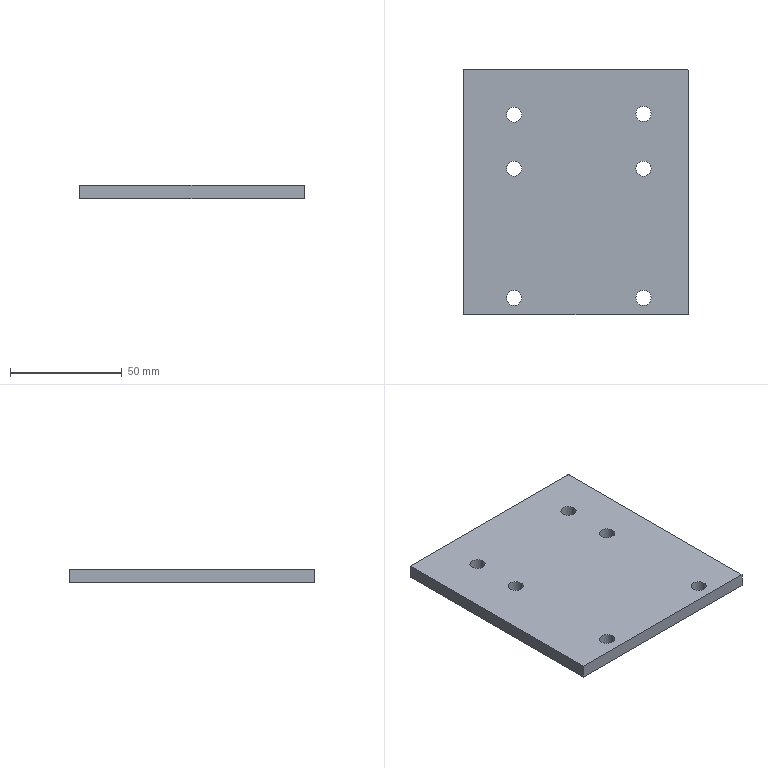Part | STEP file | Mirrored pad plate | 1 solid | 31 faces | box 100.5 x 110 x 6 mm | volume 64996 mm3 | cylinder 13 | cone 12 | plane 6 | commonest cylinder face diameters 6.8 x12 1 x1
STEP:
#1=CARTESIAN_POINT('',(238.4,0.,-5.375));
#2=VERTEX_POINT('',#1);
#3=CARTESIAN_POINT('',(231.6,0.,-5.375));
#4=VERTEX_POINT('',#3);
#5=CARTESIAN_POINT('',(235.,0.,-5.375));
#6=DIRECTION('',(0.,0.,1.));
#7=DIRECTION('',(1.,0.,0.));
#8=AXIS2_PLACEMENT_3D('',#5,#6,#7);
#9=CIRCLE('',#8,3.4);
#10=EDGE_CURVE('',#2,#4,#9,.T.);
#11=ORIENTED_EDGE('',*,*,#10,.T.);
#12=CARTESIAN_POINT('',(230.975,0.,-6.));
#13=VERTEX_POINT('',#12);
#14=CARTESIAN_POINT('',(230.975,0.,-6.));
#15=DIRECTION('',(-0.7071,0.,-0.7071));
#16=VECTOR('',#15,1000.);
#17=LINE('',#14,#16);
#18=EDGE_CURVE('',#4,#13,#17,.T.);
#19=ORIENTED_EDGE('',*,*,#18,.T.);
#20=CARTESIAN_POINT('',(239.025,0.,-6.));
#21=VERTEX_POINT('',#20);
#22=CARTESIAN_POINT('',(235.,0.,-6.));
#23=DIRECTION('',(0.,0.,1.));
#24=DIRECTION('',(1.,0.,0.));
#25=AXIS2_PLACEMENT_3D('',#22,#23,#24);
#26=CIRCLE('',#25,4.025);
#27=EDGE_CURVE('',#21,#13,#26,.T.);
#28=ORIENTED_EDGE('',*,*,#27,.F.);
#29=CARTESIAN_POINT('',(239.025,0.,-6.));
#30=DIRECTION('',(0.7071,0.,-0.7071));
#31=VECTOR('',#30,1000.);
#32=LINE('',#29,#31);
#33=EDGE_CURVE('',#2,#21,#32,.T.);
#34=ORIENTED_EDGE('',*,*,#33,.F.);
#35=EDGE_LOOP('',(#11,#19,#28,#34));
#36=FACE_OUTER_BOUND('',#35,.T.);
#37=CARTESIAN_POINT('',(235.,0.,-6.));
#38=DIRECTION('',(0.,0.,-1.));
#39=DIRECTION('',(1.,0.,0.));
#40=AXIS2_PLACEMENT_3D('',#37,#38,#39);
#41=CONICAL_SURFACE('',#40,4.025,0.7854);
#42=ADVANCED_FACE('',(#36),#41,.F.);
#43=CARTESIAN_POINT('',(231.6,0.,0.));
#44=VERTEX_POINT('',#43);
#45=CARTESIAN_POINT('',(238.4,0.,0.));
#46=VERTEX_POINT('',#45);
#47=CARTESIAN_POINT('',(235.,0.,0.));
#48=DIRECTION('',(0.,0.,-1.));
#49=DIRECTION('',(-1.,0.,0.));
#50=AXIS2_PLACEMENT_3D('',#47,#48,#49);
#51=CIRCLE('',#50,3.4);
#52=EDGE_CURVE('',#44,#46,#51,.T.);
#53=ORIENTED_EDGE('',*,*,#52,.F.);
#54=CARTESIAN_POINT('',(231.6,0.,-6.));
#55=DIRECTION('',(0.,0.,-1.));
#56=VECTOR('',#55,1000.);
#57=LINE('',#54,#56);
#58=EDGE_CURVE('',#44,#4,#57,.T.);
#59=ORIENTED_EDGE('',*,*,#58,.T.);
#60=ORIENTED_EDGE('',*,*,#10,.F.);
#61=CARTESIAN_POINT('',(238.4,0.,-6.));
#62=DIRECTION('',(0.,0.,-1.));
#63=VECTOR('',#62,1000.);
#64=LINE('',#61,#63);
#65=EDGE_CURVE('',#46,#2,#64,.T.);
#66=ORIENTED_EDGE('',*,*,#65,.F.);
#67=EDGE_LOOP('',(#53,#59,#60,#66));
#68=FACE_OUTER_BOUND('',#67,.T.);
#69=CARTESIAN_POINT('',(235.,0.,-6.));
#70=DIRECTION('',(0.,0.,-1.));
#71=DIRECTION('',(1.,0.,0.));
#72=AXIS2_PLACEMENT_3D('',#69,#70,#71);
#73=CYLINDRICAL_SURFACE('',#72,3.4);
#74=ADVANCED_FACE('',(#68),#73,.F.);
#75=CARTESIAN_POINT('',(238.4,-24.5,-5.375));
#76=VERTEX_POINT('',#75);
#77=CARTESIAN_POINT('',(231.6,-24.5,-5.375));
#78=VERTEX_POINT('',#77);
#79=CARTESIAN_POINT('',(235.,-24.5,-5.375));
#80=DIRECTION('',(0.,0.,1.));
#81=DIRECTION('',(1.,0.,0.));
#82=AXIS2_PLACEMENT_3D('',#79,#80,#81);
#83=CIRCLE('',#82,3.4);
#84=EDGE_CURVE('',#76,#78,#83,.T.);
#85=ORIENTED_EDGE('',*,*,#84,.T.);
#86=CARTESIAN_POINT('',(230.975,-24.5,-6.));
#87=VERTEX_POINT('',#86);
#88=CARTESIAN_POINT('',(230.975,-24.5,-6.));
#89=DIRECTION('',(-0.7071,0.,-0.7071));
#90=VECTOR('',#89,1000.);
#91=LINE('',#88,#90);
#92=EDGE_CURVE('',#78,#87,#91,.T.);
#93=ORIENTED_EDGE('',*,*,#92,.T.);
#94=CARTESIAN_POINT('',(239.025,-24.5,-6.));
#95=VERTEX_POINT('',#94);
#96=CARTESIAN_POINT('',(235.,-24.5,-6.));
#97=DIRECTION('',(0.,0.,1.));
#98=DIRECTION('',(1.,0.,0.));
#99=AXIS2_PLACEMENT_3D('',#96,#97,#98);
#100=CIRCLE('',#99,4.025);
#101=EDGE_CURVE('',#95,#87,#100,.T.);
#102=ORIENTED_EDGE('',*,*,#101,.F.);
#103=CARTESIAN_POINT('',(239.025,-24.5,-6.));
#104=DIRECTION('',(0.7071,0.,-0.7071));
#105=VECTOR('',#104,1000.);
#106=LINE('',#103,#105);
#107=EDGE_CURVE('',#76,#95,#106,.T.);
#108=ORIENTED_EDGE('',*,*,#107,.F.);
#109=EDGE_LOOP('',(#85,#93,#102,#108));
#110=FACE_OUTER_BOUND('',#109,.T.);
#111=CARTESIAN_POINT('',(235.,-24.5,-6.));
#112=DIRECTION('',(0.,0.,-1.));
#113=DIRECTION('',(1.,0.,0.));
#114=AXIS2_PLACEMENT_3D('',#111,#112,#113);
#115=CONICAL_SURFACE('',#114,4.025,0.7854);
#116=ADVANCED_FACE('',(#110),#115,.F.);
#117=CARTESIAN_POINT('',(231.6,-24.5,0.));
#118=VERTEX_POINT('',#117);
#119=CARTESIAN_POINT('',(238.4,-24.5,0.));
#120=VERTEX_POINT('',#119);
#121=CARTESIAN_POINT('',(235.,-24.5,0.));
#122=DIRECTION('',(0.,0.,-1.));
#123=DIRECTION('',(-1.,0.,0.));
#124=AXIS2_PLACEMENT_3D('',#121,#122,#123);
#125=CIRCLE('',#124,3.4);
#126=EDGE_CURVE('',#118,#120,#125,.T.);
#127=ORIENTED_EDGE('',*,*,#126,.F.);
#128=CARTESIAN_POINT('',(231.6,-24.5,-6.));
#129=DIRECTION('',(0.,0.,-1.));
#130=VECTOR('',#129,1000.);
#131=LINE('',#128,#130);
#132=EDGE_CURVE('',#118,#78,#131,.T.);
#133=ORIENTED_EDGE('',*,*,#132,.T.);
#134=ORIENTED_EDGE('',*,*,#84,.F.);
#135=CARTESIAN_POINT('',(238.4,-24.5,-6.));
#136=DIRECTION('',(0.,0.,-1.));
#137=VECTOR('',#136,1000.);
#138=LINE('',#135,#137);
#139=EDGE_CURVE('',#120,#76,#138,.T.);
#140=ORIENTED_EDGE('',*,*,#139,.F.);
#141=EDGE_LOOP('',(#127,#133,#134,#140));
#142=FACE_OUTER_BOUND('',#141,.T.);
#143=CARTESIAN_POINT('',(235.,-24.5,-6.));
#144=DIRECTION('',(0.,0.,-1.));
#145=DIRECTION('',(1.,0.,0.));
#146=AXIS2_PLACEMENT_3D('',#143,#144,#145);
#147=CYLINDRICAL_SURFACE('',#146,3.4);
#148=ADVANCED_FACE('',(#142),#147,.F.);
#149=CARTESIAN_POINT('',(238.4,-82.5,-5.375));
#150=VERTEX_POINT('',#149);
#151=CARTESIAN_POINT('',(231.6,-82.5,-5.375));
#152=VERTEX_POINT('',#151);
#153=CARTESIAN_POINT('',(235.,-82.5,-5.375));
#154=DIRECTION('',(0.,0.,1.));
#155=DIRECTION('',(1.,0.,0.));
#156=AXIS2_PLACEMENT_3D('',#153,#154,#155);
#157=CIRCLE('',#156,3.4);
#158=EDGE_CURVE('',#150,#152,#157,.T.);
#159=ORIENTED_EDGE('',*,*,#158,.T.);
#160=CARTESIAN_POINT('',(230.975,-82.5,-6.));
#161=VERTEX_POINT('',#160);
#162=CARTESIAN_POINT('',(230.975,-82.5,-6.));
#163=DIRECTION('',(-0.7071,0.,-0.7071));
#164=VECTOR('',#163,1000.);
#165=LINE('',#162,#164);
#166=EDGE_CURVE('',#152,#161,#165,.T.);
#167=ORIENTED_EDGE('',*,*,#166,.T.);
#168=CARTESIAN_POINT('',(239.025,-82.5,-6.));
#169=VERTEX_POINT('',#168);
#170=CARTESIAN_POINT('',(235.,-82.5,-6.));
#171=DIRECTION('',(0.,0.,1.));
#172=DIRECTION('',(1.,0.,0.));
#173=AXIS2_PLACEMENT_3D('',#170,#171,#172);
#174=CIRCLE('',#173,4.025);
#175=EDGE_CURVE('',#169,#161,#174,.T.);
#176=ORIENTED_EDGE('',*,*,#175,.F.);
#177=CARTESIAN_POINT('',(239.025,-82.5,-6.));
#178=DIRECTION('',(0.7071,0.,-0.7071));
#179=VECTOR('',#178,1000.);
#180=LINE('',#177,#179);
#181=EDGE_CURVE('',#150,#169,#180,.T.);
#182=ORIENTED_EDGE('',*,*,#181,.F.);
#183=EDGE_LOOP('',(#159,#167,#176,#182));
#184=FACE_OUTER_BOUND('',#183,.T.);
#185=CARTESIAN_POINT('',(235.,-82.5,-6.));
#186=DIRECTION('',(0.,0.,-1.));
#187=DIRECTION('',(1.,0.,0.));
#188=AXIS2_PLACEMENT_3D('',#185,#186,#187);
#189=CONICAL_SURFACE('',#188,4.025,0.7854);
#190=ADVANCED_FACE('',(#184),#189,.F.);
#191=CARTESIAN_POINT('',(231.6,-82.5,0.));
#192=VERTEX_POINT('',#191);
#193=CARTESIAN_POINT('',(238.4,-82.5,0.));
#194=VERTEX_POINT('',#193);
#195=CARTESIAN_POINT('',(235.,-82.5,0.));
#196=DIRECTION('',(0.,0.,-1.));
#197=DIRECTION('',(-1.,0.,0.));
#198=AXIS2_PLACEMENT_3D('',#195,#196,#197);
#199=CIRCLE('',#198,3.4);
#200=EDGE_CURVE('',#192,#194,#199,.T.);
#201=ORIENTED_EDGE('',*,*,#200,.F.);
#202=CARTESIAN_POINT('',(231.6,-82.5,-6.));
#203=DIRECTION('',(0.,0.,-1.));
#204=VECTOR('',#203,1000.);
#205=LINE('',#202,#204);
#206=EDGE_CURVE('',#192,#152,#205,.T.);
#207=ORIENTED_EDGE('',*,*,#206,.T.);
#208=ORIENTED_EDGE('',*,*,#158,.F.);
#209=CARTESIAN_POINT('',(238.4,-82.5,-6.));
#210=DIRECTION('',(0.,0.,-1.));
#211=VECTOR('',#210,1000.);
#212=LINE('',#209,#211);
#213=EDGE_CURVE('',#194,#150,#212,.T.);
#214=ORIENTED_EDGE('',*,*,#213,.F.);
#215=EDGE_LOOP('',(#201,#207,#208,#214));
#216=FACE_OUTER_BOUND('',#215,.T.);
#217=CARTESIAN_POINT('',(235.,-82.5,-6.));
#218=DIRECTION('',(0.,0.,-1.));
#219=DIRECTION('',(1.,0.,0.));
#220=AXIS2_PLACEMENT_3D('',#217,#218,#219);
#221=CYLINDRICAL_SURFACE('',#220,3.4);
#222=ADVANCED_FACE('',(#216),#221,.F.);
#223=CARTESIAN_POINT('',(180.4,-82.5,-5.375));
#224=VERTEX_POINT('',#223);
#225=CARTESIAN_POINT('',(173.6,-82.5,-5.375));
#226=VERTEX_POINT('',#225);
#227=CARTESIAN_POINT('',(177.,-82.5,-5.375));
#228=DIRECTION('',(0.,0.,1.));
#229=DIRECTION('',(1.,0.,0.));
#230=AXIS2_PLACEMENT_3D('',#227,#228,#229);
#231=CIRCLE('',#230,3.4);
#232=EDGE_CURVE('',#224,#226,#231,.T.);
#233=ORIENTED_EDGE('',*,*,#232,.T.);
#234=CARTESIAN_POINT('',(172.975,-82.5,-6.));
#235=VERTEX_POINT('',#234);
#236=CARTESIAN_POINT('',(172.975,-82.5,-6.));
#237=DIRECTION('',(-0.7071,0.,-0.7071));
#238=VECTOR('',#237,1000.);
#239=LINE('',#236,#238);
#240=EDGE_CURVE('',#226,#235,#239,.T.);
#241=ORIENTED_EDGE('',*,*,#240,.T.);
#242=CARTESIAN_POINT('',(181.025,-82.5,-6.));
#243=VERTEX_POINT('',#242);
#244=CARTESIAN_POINT('',(177.,-82.5,-6.));
#245=DIRECTION('',(0.,0.,1.));
#246=DIRECTION('',(1.,0.,0.));
#247=AXIS2_PLACEMENT_3D('',#244,#245,#246);
#248=CIRCLE('',#247,4.025);
#249=EDGE_CURVE('',#243,#235,#248,.T.);
#250=ORIENTED_EDGE('',*,*,#249,.F.);
#251=CARTESIAN_POINT('',(181.025,-82.5,-6.));
#252=DIRECTION('',(0.7071,0.,-0.7071));
#253=VECTOR('',#252,1000.);
#254=LINE('',#251,#253);
#255=EDGE_CURVE('',#224,#243,#254,.T.);
#256=ORIENTED_EDGE('',*,*,#255,.F.);
#257=EDGE_LOOP('',(#233,#241,#250,#256));
#258=FACE_OUTER_BOUND('',#257,.T.);
#259=CARTESIAN_POINT('',(177.,-82.5,-6.));
#260=DIRECTION('',(0.,0.,-1.));
#261=DIRECTION('',(1.,0.,0.));
#262=AXIS2_PLACEMENT_3D('',#259,#260,#261);
#263=CONICAL_SURFACE('',#262,4.025,0.7854);
#264=ADVANCED_FACE('',(#258),#263,.F.);
#265=CARTESIAN_POINT('',(173.6,-82.5,0.));
#266=VERTEX_POINT('',#265);
#267=CARTESIAN_POINT('',(180.4,-82.5,0.));
#268=VERTEX_POINT('',#267);
#269=CARTESIAN_POINT('',(177.,-82.5,0.));
#270=DIRECTION('',(0.,0.,-1.));
#271=DIRECTION('',(-1.,0.,0.));
#272=AXIS2_PLACEMENT_3D('',#269,#270,#271);
#273=CIRCLE('',#272,3.4);
#274=EDGE_CURVE('',#266,#268,#273,.T.);
#275=ORIENTED_EDGE('',*,*,#274,.F.);
#276=CARTESIAN_POINT('',(173.6,-82.5,-6.));
#277=DIRECTION('',(0.,0.,-1.));
#278=VECTOR('',#277,1000.);
#279=LINE('',#276,#278);
#280=EDGE_CURVE('',#266,#226,#279,.T.);
#281=ORIENTED_EDGE('',*,*,#280,.T.);
#282=ORIENTED_EDGE('',*,*,#232,.F.);
#283=CARTESIAN_POINT('',(180.4,-82.5,-6.));
#284=DIRECTION('',(0.,0.,-1.));
#285=VECTOR('',#284,1000.);
#286=LINE('',#283,#285);
#287=EDGE_CURVE('',#268,#224,#286,.T.);
#288=ORIENTED_EDGE('',*,*,#287,.F.);
#289=EDGE_LOOP('',(#275,#281,#282,#288));
#290=FACE_OUTER_BOUND('',#289,.T.);
#291=CARTESIAN_POINT('',(177.,-82.5,-6.));
#292=DIRECTION('',(0.,0.,-1.));
#293=DIRECTION('',(1.,0.,0.));
#294=AXIS2_PLACEMENT_3D('',#291,#292,#293);
#295=CYLINDRICAL_SURFACE('',#294,3.4);
#296=ADVANCED_FACE('',(#290),#295,.F.);
#297=CARTESIAN_POINT('',(180.4,-24.5,-5.375));
#298=VERTEX_POINT('',#297);
#299=CARTESIAN_POINT('',(173.6,-24.5,-5.375));
#300=VERTEX_POINT('',#299);
#301=CARTESIAN_POINT('',(177.,-24.5,-5.375));
#302=DIRECTION('',(0.,0.,1.));
#303=DIRECTION('',(1.,0.,0.));
#304=AXIS2_PLACEMENT_3D('',#301,#302,#303);
#305=CIRCLE('',#304,3.4);
#306=EDGE_CURVE('',#298,#300,#305,.T.);
#307=ORIENTED_EDGE('',*,*,#306,.T.);
#308=CARTESIAN_POINT('',(172.975,-24.5,-6.));
#309=VERTEX_POINT('',#308);
#310=CARTESIAN_POINT('',(172.975,-24.5,-6.));
#311=DIRECTION('',(-0.7071,0.,-0.7071));
#312=VECTOR('',#311,1000.);
#313=LINE('',#310,#312);
#314=EDGE_CURVE('',#300,#309,#313,.T.);
#315=ORIENTED_EDGE('',*,*,#314,.T.);
#316=CARTESIAN_POINT('',(181.025,-24.5,-6.));
#317=VERTEX_POINT('',#316);
#318=CARTESIAN_POINT('',(177.,-24.5,-6.));
#319=DIRECTION('',(0.,0.,1.));
#320=DIRECTION('',(1.,0.,0.));
#321=AXIS2_PLACEMENT_3D('',#318,#319,#320);
#322=CIRCLE('',#321,4.025);
#323=EDGE_CURVE('',#317,#309,#322,.T.);
#324=ORIENTED_EDGE('',*,*,#323,.F.);
#325=CARTESIAN_POINT('',(181.025,-24.5,-6.));
#326=DIRECTION('',(0.7071,0.,-0.7071));
#327=VECTOR('',#326,1000.);
#328=LINE('',#325,#327);
#329=EDGE_CURVE('',#298,#317,#328,.T.);
#330=ORIENTED_EDGE('',*,*,#329,.F.);
#331=EDGE_LOOP('',(#307,#315,#324,#330));
#332=FACE_OUTER_BOUND('',#331,.T.);
#333=CARTESIAN_POINT('',(177.,-24.5,-6.));
#334=DIRECTION('',(0.,0.,-1.));
#335=DIRECTION('',(1.,0.,0.));
#336=AXIS2_PLACEMENT_3D('',#333,#334,#335);
#337=CONICAL_SURFACE('',#336,4.025,0.7854);
#338=ADVANCED_FACE('',(#332),#337,.F.);
#339=CARTESIAN_POINT('',(173.6,-24.5,0.));
#340=VERTEX_POINT('',#339);
#341=CARTESIAN_POINT('',(180.4,-24.5,0.));
#342=VERTEX_POINT('',#341);
#343=CARTESIAN_POINT('',(177.,-24.5,0.));
#344=DIRECTION('',(0.,0.,-1.));
#345=DIRECTION('',(-1.,0.,0.));
#346=AXIS2_PLACEMENT_3D('',#343,#344,#345);
#347=CIRCLE('',#346,3.4);
#348=EDGE_CURVE('',#340,#342,#347,.T.);
#349=ORIENTED_EDGE('',*,*,#348,.F.);
#350=CARTESIAN_POINT('',(173.6,-24.5,-6.));
#351=DIRECTION('',(0.,0.,-1.));
#352=VECTOR('',#351,1000.);
#353=LINE('',#350,#352);
#354=EDGE_CURVE('',#340,#300,#353,.T.);
#355=ORIENTED_EDGE('',*,*,#354,.T.);
#356=ORIENTED_EDGE('',*,*,#306,.F.);
#357=CARTESIAN_POINT('',(180.4,-24.5,-6.));
#358=DIRECTION('',(0.,0.,-1.));
#359=VECTOR('',#358,1000.);
#360=LINE('',#357,#359);
#361=EDGE_CURVE('',#342,#298,#360,.T.);
#362=ORIENTED_EDGE('',*,*,#361,.F.);
#363=EDGE_LOOP('',(#349,#355,#356,#362));
#364=FACE_OUTER_BOUND('',#363,.T.);
#365=CARTESIAN_POINT('',(177.,-24.5,-6.));
#366=DIRECTION('',(0.,0.,-1.));
#367=DIRECTION('',(1.,0.,0.));
#368=AXIS2_PLACEMENT_3D('',#365,#366,#367);
#369=CYLINDRICAL_SURFACE('',#368,3.4);
#370=ADVANCED_FACE('',(#364),#369,.F.);
#371=CARTESIAN_POINT('',(180.4,-0.3,-5.375));
#372=VERTEX_POINT('',#371);
#373=CARTESIAN_POINT('',(173.6,-0.3,-5.375));
#374=VERTEX_POINT('',#373);
#375=CARTESIAN_POINT('',(177.,-0.3,-5.375));
#376=DIRECTION('',(0.,0.,1.));
#377=DIRECTION('',(1.,0.,0.));
#378=AXIS2_PLACEMENT_3D('',#375,#376,#377);
#379=CIRCLE('',#378,3.4);
#380=EDGE_CURVE('',#372,#374,#379,.T.);
#381=ORIENTED_EDGE('',*,*,#380,.T.);
#382=CARTESIAN_POINT('',(172.975,-0.3,-6.));
#383=VERTEX_POINT('',#382);
#384=CARTESIAN_POINT('',(172.975,-0.3,-6.));
#385=DIRECTION('',(-0.7071,0.,-0.7071));
#386=VECTOR('',#385,1000.);
#387=LINE('',#384,#386);
#388=EDGE_CURVE('',#374,#383,#387,.T.);
#389=ORIENTED_EDGE('',*,*,#388,.T.);
#390=CARTESIAN_POINT('',(181.025,-0.3,-6.));
#391=VERTEX_POINT('',#390);
#392=CARTESIAN_POINT('',(177.,-0.3,-6.));
#393=DIRECTION('',(0.,0.,1.));
#394=DIRECTION('',(1.,0.,0.));
#395=AXIS2_PLACEMENT_3D('',#392,#393,#394);
#396=CIRCLE('',#395,4.025);
#397=EDGE_CURVE('',#391,#383,#396,.T.);
#398=ORIENTED_EDGE('',*,*,#397,.F.);
#399=CARTESIAN_POINT('',(181.025,-0.3,-6.));
#400=DIRECTION('',(0.7071,0.,-0.7071));
#401=VECTOR('',#400,1000.);
#402=LINE('',#399,#401);
#403=EDGE_CURVE('',#372,#391,#402,.T.);
#404=ORIENTED_EDGE('',*,*,#403,.F.);
#405=EDGE_LOOP('',(#381,#389,#398,#404));
#406=FACE_OUTER_BOUND('',#405,.T.);
#407=CARTESIAN_POINT('',(177.,-0.3,-6.));
#408=DIRECTION('',(0.,0.,-1.));
#409=DIRECTION('',(1.,0.,0.));
#410=AXIS2_PLACEMENT_3D('',#407,#408,#409);
#411=CONICAL_SURFACE('',#410,4.025,0.7854);
#412=ADVANCED_FACE('',(#406),#411,.F.);
#413=CARTESIAN_POINT('',(173.6,-0.3,0.));
#414=VERTEX_POINT('',#413);
#415=CARTESIAN_POINT('',(180.4,-0.3,0.));
#416=VERTEX_POINT('',#415);
#417=CARTESIAN_POINT('',(177.,-0.3,0.));
#418=DIRECTION('',(0.,0.,-1.));
#419=DIRECTION('',(-1.,0.,0.));
#420=AXIS2_PLACEMENT_3D('',#417,#418,#419);
#421=CIRCLE('',#420,3.4);
#422=EDGE_CURVE('',#414,#416,#421,.T.);
#423=ORIENTED_EDGE('',*,*,#422,.F.);
#424=CARTESIAN_POINT('',(173.6,-0.3,-6.));
#425=DIRECTION('',(0.,0.,-1.));
#426=VECTOR('',#425,1000.);
#427=LINE('',#424,#426);
#428=EDGE_CURVE('',#414,#374,#427,.T.);
#429=ORIENTED_EDGE('',*,*,#428,.T.);
#430=ORIENTED_EDGE('',*,*,#380,.F.);
#431=CARTESIAN_POINT('',(180.4,-0.3,-6.));
#432=DIRECTION('',(0.,0.,-1.));
#433=VECTOR('',#432,1000.);
#434=LINE('',#431,#433);
#435=EDGE_CURVE('',#416,#372,#434,.T.);
#436=ORIENTED_EDGE('',*,*,#435,.F.);
#437=EDGE_LOOP('',(#423,#429,#430,#436));
#438=FACE_OUTER_BOUND('',#437,.T.);
#439=CARTESIAN_POINT('',(177.,-0.3,-6.));
#440=DIRECTION('',(0.,0.,-1.));
#441=DIRECTION('',(1.,0.,0.));
#442=AXIS2_PLACEMENT_3D('',#439,#440,#441);
#443=CYLINDRICAL_SURFACE('',#442,3.4);
#444=ADVANCED_FACE('',(#438),#443,.F.);
#445=CARTESIAN_POINT('',(154.5,20.,-6.));
#446=VERTEX_POINT('',#445);
#447=CARTESIAN_POINT('',(154.5,-90.,-6.));
#448=VERTEX_POINT('',#447);
#449=CARTESIAN_POINT('',(154.5,20.,-6.));
#450=DIRECTION('',(0.,-1.,0.));
#451=VECTOR('',#450,1000.);
#452=LINE('',#449,#451);
#453=EDGE_CURVE('',#446,#448,#452,.T.);
#454=ORIENTED_EDGE('',*,*,#453,.F.);
#455=CARTESIAN_POINT('',(254.5,20.,-6.));
#456=VERTEX_POINT('',#455);
#457=CARTESIAN_POINT('',(254.5,20.,-6.));
#458=DIRECTION('',(-1.,0.,0.));
#459=VECTOR('',#458,1000.);
#460=LINE('',#457,#459);
#461=EDGE_CURVE('',#456,#446,#460,.T.);
#462=ORIENTED_EDGE('',*,*,#461,.F.);
#463=CARTESIAN_POINT('',(255.,19.5,-6.));
#464=VERTEX_POINT('',#463);
#465=CARTESIAN_POINT('',(254.5,19.5,-6.));
#466=DIRECTION('',(0.,0.,1.));
#467=DIRECTION('',(-1.,0.,0.));
#468=AXIS2_PLACEMENT_3D('',#465,#466,#467);
#469=CIRCLE('',#468,0.5);
#470=EDGE_CURVE('',#464,#456,#469,.T.);
#471=ORIENTED_EDGE('',*,*,#470,.F.);
#472=CARTESIAN_POINT('',(255.,-90.,-6.));
#473=VERTEX_POINT('',#472);
#474=CARTESIAN_POINT('',(255.,19.5,-6.));
#475=DIRECTION('',(0.,1.,0.));
#476=VECTOR('',#475,1000.);
#477=LINE('',#474,#476);
#478=EDGE_CURVE('',#473,#464,#477,.T.);
#479=ORIENTED_EDGE('',*,*,#478,.F.);
#480=CARTESIAN_POINT('',(255.,-90.,-6.));
#481=DIRECTION('',(1.,0.,0.));
#482=VECTOR('',#481,1000.);
#483=LINE('',#480,#482);
#484=EDGE_CURVE('',#448,#473,#483,.T.);
#485=ORIENTED_EDGE('',*,*,#484,.F.);
#486=EDGE_LOOP('',(#454,#462,#471,#479,#485));
#487=FACE_OUTER_BOUND('',#486,.T.);
#488=ORIENTED_EDGE('',*,*,#397,.T.);
#489=CARTESIAN_POINT('',(177.,-0.3,-6.));
#490=DIRECTION('',(0.,0.,1.));
#491=DIRECTION('',(1.,0.,0.));
#492=AXIS2_PLACEMENT_3D('',#489,#490,#491);
#493=CIRCLE('',#492,4.025);
#494=EDGE_CURVE('',#383,#391,#493,.T.);
#495=ORIENTED_EDGE('',*,*,#494,.T.);
#496=EDGE_LOOP('',(#488,#495));
#497=FACE_BOUND('',#496,.T.);
#498=ORIENTED_EDGE('',*,*,#323,.T.);
#499=CARTESIAN_POINT('',(177.,-24.5,-6.));
#500=DIRECTION('',(0.,0.,1.));
#501=DIRECTION('',(1.,0.,0.));
#502=AXIS2_PLACEMENT_3D('',#499,#500,#501);
#503=CIRCLE('',#502,4.025);
#504=EDGE_CURVE('',#309,#317,#503,.T.);
#505=ORIENTED_EDGE('',*,*,#504,.T.);
#506=EDGE_LOOP('',(#498,#505));
#507=FACE_BOUND('',#506,.T.);
#508=ORIENTED_EDGE('',*,*,#249,.T.);
#509=CARTESIAN_POINT('',(177.,-82.5,-6.));
#510=DIRECTION('',(0.,0.,1.));
#511=DIRECTION('',(1.,0.,0.));
#512=AXIS2_PLACEMENT_3D('',#509,#510,#511);
#513=CIRCLE('',#512,4.025);
#514=EDGE_CURVE('',#235,#243,#513,.T.);
#515=ORIENTED_EDGE('',*,*,#514,.T.);
#516=EDGE_LOOP('',(#508,#515));
#517=FACE_BOUND('',#516,.T.);
#518=ORIENTED_EDGE('',*,*,#175,.T.);
#519=CARTESIAN_POINT('',(235.,-82.5,-6.));
#520=DIRECTION('',(0.,0.,1.));
#521=DIRECTION('',(1.,0.,0.));
#522=AXIS2_PLACEMENT_3D('',#519,#520,#521);
#523=CIRCLE('',#522,4.025);
#524=EDGE_CURVE('',#161,#169,#523,.T.);
#525=ORIENTED_EDGE('',*,*,#524,.T.);
#526=EDGE_LOOP('',(#518,#525));
#527=FACE_BOUND('',#526,.T.);
#528=ORIENTED_EDGE('',*,*,#101,.T.);
#529=CARTESIAN_POINT('',(235.,-24.5,-6.));
#530=DIRECTION('',(0.,0.,1.));
#531=DIRECTION('',(1.,0.,0.));
#532=AXIS2_PLACEMENT_3D('',#529,#530,#531);
#533=CIRCLE('',#532,4.025);
#534=EDGE_CURVE('',#87,#95,#533,.T.);
#535=ORIENTED_EDGE('',*,*,#534,.T.);
#536=EDGE_LOOP('',(#528,#535));
#537=FACE_BOUND('',#536,.T.);
#538=ORIENTED_EDGE('',*,*,#27,.T.);
#539=CARTESIAN_POINT('',(235.,0.,-6.));
#540=DIRECTION('',(0.,0.,1.));
#541=DIRECTION('',(1.,0.,0.));
#542=AXIS2_PLACEMENT_3D('',#539,#540,#541);
#543=CIRCLE('',#542,4.025);
#544=EDGE_CURVE('',#13,#21,#543,.T.);
#545=ORIENTED_EDGE('',*,*,#544,.T.);
#546=EDGE_LOOP('',(#538,#545));
#547=FACE_BOUND('',#546,.T.);
#548=CARTESIAN_POINT('',(254.5,19.5,-6.));
#549=DIRECTION('',(0.,0.,1.));
#550=DIRECTION('',(-1.,0.,0.));
#551=AXIS2_PLACEMENT_3D('',#548,#549,#550);
#552=PLANE('',#551);
#553=ADVANCED_FACE('',(#487,#497,#507,#517,#527,#537,#547),#552,.F.);
#554=CARTESIAN_POINT('',(154.5,20.,0.));
#555=VERTEX_POINT('',#554);
#556=CARTESIAN_POINT('',(154.5,-90.,0.));
#557=VERTEX_POINT('',#556);
#558=CARTESIAN_POINT('',(154.5,20.,0.));
#559=DIRECTION('',(0.,-1.,0.));
#560=VECTOR('',#559,1000.);
#561=LINE('',#558,#560);
#562=EDGE_CURVE('',#555,#557,#561,.T.);
#563=ORIENTED_EDGE('',*,*,#562,.F.);
#564=CARTESIAN_POINT('',(154.5,20.,-6.));
#565=DIRECTION('',(0.,0.,1.));
#566=VECTOR('',#565,1000.);
#567=LINE('',#564,#566);
#568=EDGE_CURVE('',#446,#555,#567,.T.);
#569=ORIENTED_EDGE('',*,*,#568,.F.);
#570=ORIENTED_EDGE('',*,*,#453,.T.);
#571=CARTESIAN_POINT('',(154.5,-90.,-6.));
#572=DIRECTION('',(0.,0.,1.));
#573=VECTOR('',#572,1000.);
#574=LINE('',#571,#573);
#575=EDGE_CURVE('',#448,#557,#574,.T.);
#576=ORIENTED_EDGE('',*,*,#575,.T.);
#577=EDGE_LOOP('',(#563,#569,#570,#576));
#578=FACE_OUTER_BOUND('',#577,.T.);
#579=CARTESIAN_POINT('',(154.5,20.,-6.));
#580=DIRECTION('',(1.,0.,0.));
#581=DIRECTION('',(0.,1.,0.));
#582=AXIS2_PLACEMENT_3D('',#579,#580,#581);
#583=PLANE('',#582);
#584=ADVANCED_FACE('',(#578),#583,.F.);
#585=CARTESIAN_POINT('',(255.,-90.,0.));
#586=VERTEX_POINT('',#585);
#587=CARTESIAN_POINT('',(255.,-90.,0.));
#588=DIRECTION('',(1.,0.,0.));
#589=VECTOR('',#588,1000.);
#590=LINE('',#587,#589);
#591=EDGE_CURVE('',#557,#586,#590,.T.);
#592=ORIENTED_EDGE('',*,*,#591,.F.);
#593=ORIENTED_EDGE('',*,*,#575,.F.);
#594=ORIENTED_EDGE('',*,*,#484,.T.);
#595=CARTESIAN_POINT('',(255.,-90.,-6.));
#596=DIRECTION('',(0.,0.,1.));
#597=VECTOR('',#596,1000.);
#598=LINE('',#595,#597);
#599=EDGE_CURVE('',#473,#586,#598,.T.);
#600=ORIENTED_EDGE('',*,*,#599,.T.);
#601=EDGE_LOOP('',(#592,#593,#594,#600));
#602=FACE_OUTER_BOUND('',#601,.T.);
#603=CARTESIAN_POINT('',(255.,-90.,-6.));
#604=DIRECTION('',(0.,1.,0.));
#605=DIRECTION('',(-1.,0.,0.));
#606=AXIS2_PLACEMENT_3D('',#603,#604,#605);
#607=PLANE('',#606);
#608=ADVANCED_FACE('',(#602),#607,.F.);
#609=CARTESIAN_POINT('',(255.,19.5,0.));
#610=VERTEX_POINT('',#609);
#611=CARTESIAN_POINT('',(255.,19.5,0.));
#612=DIRECTION('',(0.,1.,0.));
#613=VECTOR('',#612,1000.);
#614=LINE('',#611,#613);
#615=EDGE_CURVE('',#586,#610,#614,.T.);
#616=ORIENTED_EDGE('',*,*,#615,.F.);
#617=ORIENTED_EDGE('',*,*,#599,.F.);
#618=ORIENTED_EDGE('',*,*,#478,.T.);
#619=CARTESIAN_POINT('',(255.,19.5,-6.));
#620=DIRECTION('',(0.,0.,1.));
#621=VECTOR('',#620,1000.);
#622=LINE('',#619,#621);
#623=EDGE_CURVE('',#464,#610,#622,.T.);
#624=ORIENTED_EDGE('',*,*,#623,.T.);
#625=EDGE_LOOP('',(#616,#617,#618,#624));
#626=FACE_OUTER_BOUND('',#625,.T.);
#627=CARTESIAN_POINT('',(255.,19.5,-6.));
#628=DIRECTION('',(-1.,0.,0.));
#629=DIRECTION('',(0.,0.,-1.));
#630=AXIS2_PLACEMENT_3D('',#627,#628,#629);
#631=PLANE('',#630);
#632=ADVANCED_FACE('',(#626),#631,.F.);
#633=CARTESIAN_POINT('',(254.5,20.,0.));
#634=VERTEX_POINT('',#633);
#635=CARTESIAN_POINT('',(254.5,19.5,0.));
#636=DIRECTION('',(0.,0.,1.));
#637=DIRECTION('',(-1.,0.,0.));
#638=AXIS2_PLACEMENT_3D('',#635,#636,#637);
#639=CIRCLE('',#638,0.5);
#640=EDGE_CURVE('',#610,#634,#639,.T.);
#641=ORIENTED_EDGE('',*,*,#640,.F.);
#642=ORIENTED_EDGE('',*,*,#623,.F.);
#643=ORIENTED_EDGE('',*,*,#470,.T.);
#644=CARTESIAN_POINT('',(254.5,20.,-6.));
#645=DIRECTION('',(0.,0.,1.));
#646=VECTOR('',#645,1000.);
#647=LINE('',#644,#646);
#648=EDGE_CURVE('',#456,#634,#647,.T.);
#649=ORIENTED_EDGE('',*,*,#648,.T.);
#650=EDGE_LOOP('',(#641,#642,#643,#649));
#651=FACE_OUTER_BOUND('',#650,.T.);
#652=CARTESIAN_POINT('',(254.5,19.5,-6.));
#653=DIRECTION('',(0.,0.,1.));
#654=DIRECTION('',(-1.,0.,0.));
#655=AXIS2_PLACEMENT_3D('',#652,#653,#654);
#656=CYLINDRICAL_SURFACE('',#655,0.5);
#657=ADVANCED_FACE('',(#651),#656,.T.);
#658=CARTESIAN_POINT('',(254.5,20.,0.));
#659=DIRECTION('',(-1.,0.,0.));
#660=VECTOR('',#659,1000.);
#661=LINE('',#658,#660);
#662=EDGE_CURVE('',#634,#555,#661,.T.);
#663=ORIENTED_EDGE('',*,*,#662,.F.);
#664=ORIENTED_EDGE('',*,*,#648,.F.);
#665=ORIENTED_EDGE('',*,*,#461,.T.);
#666=ORIENTED_EDGE('',*,*,#568,.T.);
#667=EDGE_LOOP('',(#663,#664,#665,#666));
#668=FACE_OUTER_BOUND('',#667,.T.);
#669=CARTESIAN_POINT('',(254.5,20.,-6.));
#670=DIRECTION('',(0.,-1.,0.));
#671=DIRECTION('',(1.,0.,0.));
#672=AXIS2_PLACEMENT_3D('',#669,#670,#671);
#673=PLANE('',#672);
#674=ADVANCED_FACE('',(#668),#673,.F.);
#675=CARTESIAN_POINT('',(235.,0.,0.));
#676=DIRECTION('',(0.,0.,-1.));
#677=DIRECTION('',(-1.,0.,0.));
#678=AXIS2_PLACEMENT_3D('',#675,#676,#677);
#679=CIRCLE('',#678,3.4);
#680=EDGE_CURVE('',#46,#44,#679,.T.);
#681=ORIENTED_EDGE('',*,*,#680,.T.);
#682=ORIENTED_EDGE('',*,*,#52,.T.);
#683=EDGE_LOOP('',(#681,#682));
#684=FACE_BOUND('',#683,.T.);
#685=CARTESIAN_POINT('',(235.,-24.5,0.));
#686=DIRECTION('',(0.,0.,-1.));
#687=DIRECTION('',(-1.,0.,0.));
#688=AXIS2_PLACEMENT_3D('',#685,#686,#687);
#689=CIRCLE('',#688,3.4);
#690=EDGE_CURVE('',#120,#118,#689,.T.);
#691=ORIENTED_EDGE('',*,*,#690,.T.);
#692=ORIENTED_EDGE('',*,*,#126,.T.);
#693=EDGE_LOOP('',(#691,#692));
#694=FACE_BOUND('',#693,.T.);
#695=CARTESIAN_POINT('',(235.,-82.5,0.));
#696=DIRECTION('',(0.,0.,-1.));
#697=DIRECTION('',(-1.,0.,0.));
#698=AXIS2_PLACEMENT_3D('',#695,#696,#697);
#699=CIRCLE('',#698,3.4);
#700=EDGE_CURVE('',#194,#192,#699,.T.);
#701=ORIENTED_EDGE('',*,*,#700,.T.);
#702=ORIENTED_EDGE('',*,*,#200,.T.);
#703=EDGE_LOOP('',(#701,#702));
#704=FACE_BOUND('',#703,.T.);
#705=CARTESIAN_POINT('',(177.,-82.5,0.));
#706=DIRECTION('',(0.,0.,-1.));
#707=DIRECTION('',(-1.,0.,0.));
#708=AXIS2_PLACEMENT_3D('',#705,#706,#707);
#709=CIRCLE('',#708,3.4);
#710=EDGE_CURVE('',#268,#266,#709,.T.);
#711=ORIENTED_EDGE('',*,*,#710,.T.);
#712=ORIENTED_EDGE('',*,*,#274,.T.);
#713=EDGE_LOOP('',(#711,#712));
#714=FACE_BOUND('',#713,.T.);
#715=CARTESIAN_POINT('',(177.,-24.5,0.));
#716=DIRECTION('',(0.,0.,-1.));
#717=DIRECTION('',(-1.,0.,0.));
#718=AXIS2_PLACEMENT_3D('',#715,#716,#717);
#719=CIRCLE('',#718,3.4);
#720=EDGE_CURVE('',#342,#340,#719,.T.);
#721=ORIENTED_EDGE('',*,*,#720,.T.);
#722=ORIENTED_EDGE('',*,*,#348,.T.);
#723=EDGE_LOOP('',(#721,#722));
#724=FACE_BOUND('',#723,.T.);
#725=CARTESIAN_POINT('',(177.,-0.3,0.));
#726=DIRECTION('',(0.,0.,-1.));
#727=DIRECTION('',(-1.,0.,0.));
#728=AXIS2_PLACEMENT_3D('',#725,#726,#727);
#729=CIRCLE('',#728,3.4);
#730=EDGE_CURVE('',#416,#414,#729,.T.);
#731=ORIENTED_EDGE('',*,*,#730,.T.);
#732=ORIENTED_EDGE('',*,*,#422,.T.);
#733=EDGE_LOOP('',(#731,#732));
#734=FACE_BOUND('',#733,.T.);
#735=ORIENTED_EDGE('',*,*,#562,.T.);
#736=ORIENTED_EDGE('',*,*,#591,.T.);
#737=ORIENTED_EDGE('',*,*,#615,.T.);
#738=ORIENTED_EDGE('',*,*,#640,.T.);
#739=ORIENTED_EDGE('',*,*,#662,.T.);
#740=EDGE_LOOP('',(#735,#736,#737,#738,#739));
#741=FACE_OUTER_BOUND('',#740,.T.);
#742=CARTESIAN_POINT('',(254.5,19.5,0.));
#743=DIRECTION('',(0.,0.,1.));
#744=DIRECTION('',(-1.,0.,0.));
#745=AXIS2_PLACEMENT_3D('',#742,#743,#744);
#746=PLANE('',#745);
#747=ADVANCED_FACE('',(#684,#694,#704,#714,#724,#734,#741),#746,.T.);
#748=ORIENTED_EDGE('',*,*,#428,.F.);
#749=ORIENTED_EDGE('',*,*,#730,.F.);
#750=ORIENTED_EDGE('',*,*,#435,.T.);
#751=CARTESIAN_POINT('',(177.,-0.3,-5.375));
#752=DIRECTION('',(0.,0.,1.));
#753=DIRECTION('',(1.,0.,0.));
#754=AXIS2_PLACEMENT_3D('',#751,#752,#753);
#755=CIRCLE('',#754,3.4);
#756=EDGE_CURVE('',#374,#372,#755,.T.);
#757=ORIENTED_EDGE('',*,*,#756,.F.);
#758=EDGE_LOOP('',(#748,#749,#750,#757));
#759=FACE_OUTER_BOUND('',#758,.T.);
#760=CARTESIAN_POINT('',(177.,-0.3,-6.));
#761=DIRECTION('',(0.,0.,-1.));
#762=DIRECTION('',(1.,0.,0.));
#763=AXIS2_PLACEMENT_3D('',#760,#761,#762);
#764=CYLINDRICAL_SURFACE('',#763,3.4);
#765=ADVANCED_FACE('',(#759),#764,.F.);
#766=ORIENTED_EDGE('',*,*,#388,.F.);
#767=ORIENTED_EDGE('',*,*,#756,.T.);
#768=ORIENTED_EDGE('',*,*,#403,.T.);
#769=ORIENTED_EDGE('',*,*,#494,.F.);
#770=EDGE_LOOP('',(#766,#767,#768,#769));
#771=FACE_OUTER_BOUND('',#770,.T.);
#772=CARTESIAN_POINT('',(177.,-0.3,-6.));
#773=DIRECTION('',(0.,0.,-1.));
#774=DIRECTION('',(1.,0.,0.));
#775=AXIS2_PLACEMENT_3D('',#772,#773,#774);
#776=CONICAL_SURFACE('',#775,4.025,0.7854);
#777=ADVANCED_FACE('',(#771),#776,.F.);
#778=ORIENTED_EDGE('',*,*,#354,.F.);
#779=ORIENTED_EDGE('',*,*,#720,.F.);
#780=ORIENTED_EDGE('',*,*,#361,.T.);
#781=CARTESIAN_POINT('',(177.,-24.5,-5.375));
#782=DIRECTION('',(0.,0.,1.));
#783=DIRECTION('',(1.,0.,0.));
#784=AXIS2_PLACEMENT_3D('',#781,#782,#783);
#785=CIRCLE('',#784,3.4);
#786=EDGE_CURVE('',#300,#298,#785,.T.);
#787=ORIENTED_EDGE('',*,*,#786,.F.);
#788=EDGE_LOOP('',(#778,#779,#780,#787));
#789=FACE_OUTER_BOUND('',#788,.T.);
#790=CARTESIAN_POINT('',(177.,-24.5,-6.));
#791=DIRECTION('',(0.,0.,-1.));
#792=DIRECTION('',(1.,0.,0.));
#793=AXIS2_PLACEMENT_3D('',#790,#791,#792);
#794=CYLINDRICAL_SURFACE('',#793,3.4);
#795=ADVANCED_FACE('',(#789),#794,.F.);
#796=ORIENTED_EDGE('',*,*,#314,.F.);
#797=ORIENTED_EDGE('',*,*,#786,.T.);
#798=ORIENTED_EDGE('',*,*,#329,.T.);
#799=ORIENTED_EDGE('',*,*,#504,.F.);
#800=EDGE_LOOP('',(#796,#797,#798,#799));
#801=FACE_OUTER_BOUND('',#800,.T.);
#802=CARTESIAN_POINT('',(177.,-24.5,-6.));
#803=DIRECTION('',(0.,0.,-1.));
#804=DIRECTION('',(1.,0.,0.));
#805=AXIS2_PLACEMENT_3D('',#802,#803,#804);
#806=CONICAL_SURFACE('',#805,4.025,0.7854);
#807=ADVANCED_FACE('',(#801),#806,.F.);
#808=ORIENTED_EDGE('',*,*,#280,.F.);
#809=ORIENTED_EDGE('',*,*,#710,.F.);
#810=ORIENTED_EDGE('',*,*,#287,.T.);
#811=CARTESIAN_POINT('',(177.,-82.5,-5.375));
#812=DIRECTION('',(0.,0.,1.));
#813=DIRECTION('',(1.,0.,0.));
#814=AXIS2_PLACEMENT_3D('',#811,#812,#813);
#815=CIRCLE('',#814,3.4);
#816=EDGE_CURVE('',#226,#224,#815,.T.);
#817=ORIENTED_EDGE('',*,*,#816,.F.);
#818=EDGE_LOOP('',(#808,#809,#810,#817));
#819=FACE_OUTER_BOUND('',#818,.T.);
#820=CARTESIAN_POINT('',(177.,-82.5,-6.));
#821=DIRECTION('',(0.,0.,-1.));
#822=DIRECTION('',(1.,0.,0.));
#823=AXIS2_PLACEMENT_3D('',#820,#821,#822);
#824=CYLINDRICAL_SURFACE('',#823,3.4);
#825=ADVANCED_FACE('',(#819),#824,.F.);
#826=ORIENTED_EDGE('',*,*,#240,.F.);
#827=ORIENTED_EDGE('',*,*,#816,.T.);
#828=ORIENTED_EDGE('',*,*,#255,.T.);
#829=ORIENTED_EDGE('',*,*,#514,.F.);
#830=EDGE_LOOP('',(#826,#827,#828,#829));
#831=FACE_OUTER_BOUND('',#830,.T.);
#832=CARTESIAN_POINT('',(177.,-82.5,-6.));
#833=DIRECTION('',(0.,0.,-1.));
#834=DIRECTION('',(1.,0.,0.));
#835=AXIS2_PLACEMENT_3D('',#832,#833,#834);
#836=CONICAL_SURFACE('',#835,4.025,0.7854);
#837=ADVANCED_FACE('',(#831),#836,.F.);
#838=ORIENTED_EDGE('',*,*,#206,.F.);
#839=ORIENTED_EDGE('',*,*,#700,.F.);
#840=ORIENTED_EDGE('',*,*,#213,.T.);
#841=CARTESIAN_POINT('',(235.,-82.5,-5.375));
#842=DIRECTION('',(0.,0.,1.));
#843=DIRECTION('',(1.,0.,0.));
#844=AXIS2_PLACEMENT_3D('',#841,#842,#843);
#845=CIRCLE('',#844,3.4);
#846=EDGE_CURVE('',#152,#150,#845,.T.);
#847=ORIENTED_EDGE('',*,*,#846,.F.);
#848=EDGE_LOOP('',(#838,#839,#840,#847));
#849=FACE_OUTER_BOUND('',#848,.T.);
#850=CARTESIAN_POINT('',(235.,-82.5,-6.));
#851=DIRECTION('',(0.,0.,-1.));
#852=DIRECTION('',(1.,0.,0.));
#853=AXIS2_PLACEMENT_3D('',#850,#851,#852);
#854=CYLINDRICAL_SURFACE('',#853,3.4);
#855=ADVANCED_FACE('',(#849),#854,.F.);
#856=ORIENTED_EDGE('',*,*,#166,.F.);
#857=ORIENTED_EDGE('',*,*,#846,.T.);
#858=ORIENTED_EDGE('',*,*,#181,.T.);
#859=ORIENTED_EDGE('',*,*,#524,.F.);
#860=EDGE_LOOP('',(#856,#857,#858,#859));
#861=FACE_OUTER_BOUND('',#860,.T.);
#862=CARTESIAN_POINT('',(235.,-82.5,-6.));
#863=DIRECTION('',(0.,0.,-1.));
#864=DIRECTION('',(1.,0.,0.));
#865=AXIS2_PLACEMENT_3D('',#862,#863,#864);
#866=CONICAL_SURFACE('',#865,4.025,0.7854);
#867=ADVANCED_FACE('',(#861),#866,.F.);
#868=ORIENTED_EDGE('',*,*,#132,.F.);
#869=ORIENTED_EDGE('',*,*,#690,.F.);
#870=ORIENTED_EDGE('',*,*,#139,.T.);
#871=CARTESIAN_POINT('',(235.,-24.5,-5.375));
#872=DIRECTION('',(0.,0.,1.));
#873=DIRECTION('',(1.,0.,0.));
#874=AXIS2_PLACEMENT_3D('',#871,#872,#873);
#875=CIRCLE('',#874,3.4);
#876=EDGE_CURVE('',#78,#76,#875,.T.);
#877=ORIENTED_EDGE('',*,*,#876,.F.);
#878=EDGE_LOOP('',(#868,#869,#870,#877));
#879=FACE_OUTER_BOUND('',#878,.T.);
#880=CARTESIAN_POINT('',(235.,-24.5,-6.));
#881=DIRECTION('',(0.,0.,-1.));
#882=DIRECTION('',(1.,0.,0.));
#883=AXIS2_PLACEMENT_3D('',#880,#881,#882);
#884=CYLINDRICAL_SURFACE('',#883,3.4);
#885=ADVANCED_FACE('',(#879),#884,.F.);
#886=ORIENTED_EDGE('',*,*,#92,.F.);
#887=ORIENTED_EDGE('',*,*,#876,.T.);
#888=ORIENTED_EDGE('',*,*,#107,.T.);
#889=ORIENTED_EDGE('',*,*,#534,.F.);
#890=EDGE_LOOP('',(#886,#887,#888,#889));
#891=FACE_OUTER_BOUND('',#890,.T.);
#892=CARTESIAN_POINT('',(235.,-24.5,-6.));
#893=DIRECTION('',(0.,0.,-1.));
#894=DIRECTION('',(1.,0.,0.));
#895=AXIS2_PLACEMENT_3D('',#892,#893,#894);
#896=CONICAL_SURFACE('',#895,4.025,0.7854);
#897=ADVANCED_FACE('',(#891),#896,.F.);
#898=ORIENTED_EDGE('',*,*,#58,.F.);
#899=ORIENTED_EDGE('',*,*,#680,.F.);
#900=ORIENTED_EDGE('',*,*,#65,.T.);
#901=CARTESIAN_POINT('',(235.,0.,-5.375));
#902=DIRECTION('',(0.,0.,1.));
#903=DIRECTION('',(1.,0.,0.));
#904=AXIS2_PLACEMENT_3D('',#901,#902,#903);
#905=CIRCLE('',#904,3.4);
#906=EDGE_CURVE('',#4,#2,#905,.T.);
#907=ORIENTED_EDGE('',*,*,#906,.F.);
#908=EDGE_LOOP('',(#898,#899,#900,#907));
#909=FACE_OUTER_BOUND('',#908,.T.);
#910=CARTESIAN_POINT('',(235.,0.,-6.));
#911=DIRECTION('',(0.,0.,-1.));
#912=DIRECTION('',(1.,0.,0.));
#913=AXIS2_PLACEMENT_3D('',#910,#911,#912);
#914=CYLINDRICAL_SURFACE('',#913,3.4);
#915=ADVANCED_FACE('',(#909),#914,.F.);
#916=ORIENTED_EDGE('',*,*,#18,.F.);
#917=ORIENTED_EDGE('',*,*,#906,.T.);
#918=ORIENTED_EDGE('',*,*,#33,.T.);
#919=ORIENTED_EDGE('',*,*,#544,.F.);
#920=EDGE_LOOP('',(#916,#917,#918,#919));
#921=FACE_OUTER_BOUND('',#920,.T.);
#922=CARTESIAN_POINT('',(235.,0.,-6.));
#923=DIRECTION('',(0.,0.,-1.));
#924=DIRECTION('',(1.,0.,0.));
#925=AXIS2_PLACEMENT_3D('',#922,#923,#924);
#926=CONICAL_SURFACE('',#925,4.025,0.7854);
#927=ADVANCED_FACE('',(#921),#926,.F.);
#928=CLOSED_SHELL('',(#42,#74,#116,#148,#190,#222,#264,#296,#338,#370,#412,#444,#553,#584,#608,#632,#657,#674,#747,#765,#777,#795,#807,#825,#837,#855,#867,#885,#897,#915,#927));
#929=MANIFOLD_SOLID_BREP('',#928);
#930=CARTESIAN_POINT('',(0.,0.,0.));
#931=DIRECTION('',(0.,0.,1.));
#932=DIRECTION('',(1.,0.,0.));
#933=AXIS2_PLACEMENT_3D('',#930,#931,#932);
#934=(LENGTH_UNIT()NAMED_UNIT(*)SI_UNIT(.MILLI.,.METRE.));
#935=UNCERTAINTY_MEASURE_WITH_UNIT(LENGTH_MEASURE(0.00001),#934,'','');
#936=(NAMED_UNIT(*)PLANE_ANGLE_UNIT()SI_UNIT($,.RADIAN.));
#937=(NAMED_UNIT(*)SI_UNIT($,.STERADIAN.)SOLID_ANGLE_UNIT());
#938=(GEOMETRIC_REPRESENTATION_CONTEXT(3)GLOBAL_UNCERTAINTY_ASSIGNED_CONTEXT((#935))GLOBAL_UNIT_ASSIGNED_CONTEXT((#934,#936,#937))REPRESENTATION_CONTEXT('',''));
#939=ADVANCED_BREP_SHAPE_REPRESENTATION('',(#929,#933),#938);